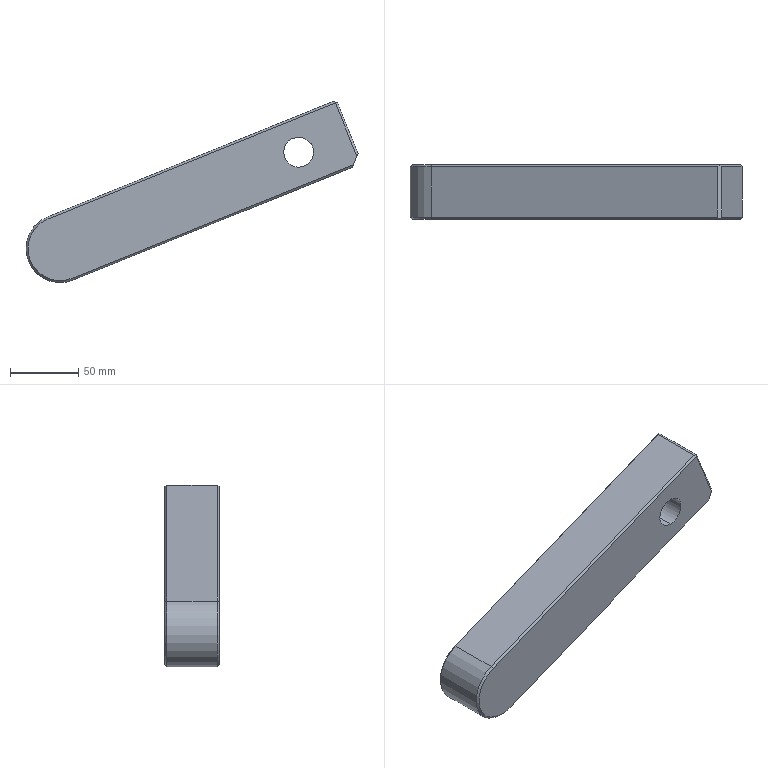Part | Creo | 1 solid | 21 faces | box 243.584 x 40 x 133.061 mm | volume 471581 mm3 | plane 14 | cylinder 5 | cone 2 | commonest cylinder face diameters 22 x2 31 x2 50 x1
STEP:
#1=CARTESIAN_POINT('',(93.939,390.,-84.108));
#2=VERTEX_POINT('',#1);
#3=CARTESIAN_POINT('',(-116.807,390.,-169.256));
#4=VERTEX_POINT('',#3);
#5=CARTESIAN_POINT('',(93.939,390.,-84.108));
#6=DIRECTION('',(-0.9272,0.,-0.3746));
#7=VECTOR('',#6,227.297);
#8=LINE('',#5,#7);
#9=EDGE_CURVE('',#2,#4,#8,.T.);
#10=ORIENTED_EDGE('',*,*,#9,.T.);
#11=CARTESIAN_POINT('',(-108.414,390.,-214.541));
#12=VERTEX_POINT('',#11);
#13=CARTESIAN_POINT('',(-108.004,390.,-191.044));
#14=DIRECTION('',(0.,1.,0.));
#15=DIRECTION('',(-0.01745,0.,-0.9998));
#16=AXIS2_PLACEMENT_3D('',#13,#14,#15);
#17=CIRCLE('',#16,23.5);
#18=EDGE_CURVE('',#12,#4,#17,.T.);
#19=ORIENTED_EDGE('',*,*,#18,.F.);
#20=CARTESIAN_POINT('',(-99.201,390.,-212.833));
#21=VERTEX_POINT('',#20);
#22=CARTESIAN_POINT('',(-108.004,390.,-191.044));
#23=DIRECTION('',(0.,1.,0.));
#24=DIRECTION('',(0.3746,0.,-0.9272));
#25=AXIS2_PLACEMENT_3D('',#22,#23,#24);
#26=CIRCLE('',#25,23.5);
#27=EDGE_CURVE('',#21,#12,#26,.T.);
#28=ORIENTED_EDGE('',*,*,#27,.F.);
#29=CARTESIAN_POINT('',(107.104,390.,-129.481));
#30=VERTEX_POINT('',#29);
#31=CARTESIAN_POINT('',(-99.201,390.,-212.833));
#32=DIRECTION('',(0.9272,0.,0.3746));
#33=VECTOR('',#32,222.507);
#34=LINE('',#31,#33);
#35=EDGE_CURVE('',#21,#30,#34,.T.);
#36=ORIENTED_EDGE('',*,*,#35,.T.);
#37=CARTESIAN_POINT('',(109.751,390.,-123.245));
#38=VERTEX_POINT('',#37);
#39=CARTESIAN_POINT('',(109.751,390.,-123.245));
#40=DIRECTION('',(-0.3907,0.,-0.9205));
#41=VECTOR('',#40,6.774);
#42=LINE('',#39,#41);
#43=EDGE_CURVE('',#38,#30,#42,.T.);
#44=ORIENTED_EDGE('',*,*,#43,.F.);
#45=CARTESIAN_POINT('',(109.751,390.,-123.245));
#46=DIRECTION('',(-0.3746,0.,0.9272));
#47=VECTOR('',#46,42.21);
#48=LINE('',#45,#47);
#49=EDGE_CURVE('',#38,#2,#48,.T.);
#50=ORIENTED_EDGE('',*,*,#49,.T.);
#51=EDGE_LOOP('',(#10,#19,#28,#36,#44,#50));
#52=FACE_OUTER_BOUND('',#51,.F.);
#53=CARTESIAN_POINT('',(67.046,390.,-135.82));
#54=VERTEX_POINT('',#53);
#55=CARTESIAN_POINT('',(67.316,390.,-104.822));
#56=VERTEX_POINT('',#55);
#57=CARTESIAN_POINT('',(67.046,390.,-120.32));
#58=DIRECTION('',(0.,-1.,0.));
#59=DIRECTION('',(0.,0.,-1.));
#60=AXIS2_PLACEMENT_3D('',#57,#58,#59);
#61=CIRCLE('',#60,15.5);
#62=EDGE_CURVE('',#54,#56,#61,.T.);
#63=ORIENTED_EDGE('',*,*,#62,.F.);
#64=CARTESIAN_POINT('',(66.775,390.,-135.817));
#65=VERTEX_POINT('',#64);
#66=CARTESIAN_POINT('',(67.046,390.,-120.32));
#67=DIRECTION('',(0.,-1.,0.));
#68=DIRECTION('',(-0.01745,0.,-0.9998));
#69=AXIS2_PLACEMENT_3D('',#66,#67,#68);
#70=CIRCLE('',#69,15.5);
#71=EDGE_CURVE('',#65,#54,#70,.T.);
#72=ORIENTED_EDGE('',*,*,#71,.F.);
#73=CARTESIAN_POINT('',(67.046,390.,-120.32));
#74=DIRECTION('',(0.,-1.,0.));
#75=DIRECTION('',(0.01745,0.,0.9998));
#76=AXIS2_PLACEMENT_3D('',#73,#74,#75);
#77=CIRCLE('',#76,15.5);
#78=EDGE_CURVE('',#56,#65,#77,.T.);
#79=ORIENTED_EDGE('',*,*,#78,.F.);
#80=EDGE_LOOP('',(#63,#72,#79));
#81=FACE_BOUND('',#80,.F.);
#82=CARTESIAN_POINT('',(343.725,390.,-2.208));
#83=DIRECTION('',(0.,1.,0.));
#84=DIRECTION('',(-0.01745,0.,-0.9998));
#85=AXIS2_PLACEMENT_3D('',#82,#83,#84);
#86=PLANE('',#85);
#87=ADVANCED_FACE('',(#52,#81),#86,.T.);
#88=CARTESIAN_POINT('',(94.157,389.605,-83.594));
#89=VERTEX_POINT('',#88);
#90=CARTESIAN_POINT('',(94.157,389.605,-83.594));
#91=DIRECTION('',(-0.319,0.5774,-0.7516));
#92=VECTOR('',#91,0.6844);
#93=LINE('',#90,#92);
#94=EDGE_CURVE('',#89,#2,#93,.T.);
#95=ORIENTED_EDGE('',*,*,#94,.F.);
#96=CARTESIAN_POINT('',(92.719,388.5,-82.984));
#97=VERTEX_POINT('',#96);
#98=CARTESIAN_POINT('',(92.719,388.5,-82.984));
#99=DIRECTION('',(0.7516,0.5774,-0.319));
#100=VECTOR('',#99,1.914);
#101=LINE('',#98,#100);
#102=EDGE_CURVE('',#97,#89,#101,.T.);
#103=ORIENTED_EDGE('',*,*,#102,.F.);
#104=CARTESIAN_POINT('',(-117.369,388.5,-167.865));
#105=VERTEX_POINT('',#104);
#106=CARTESIAN_POINT('',(-117.369,388.5,-167.865));
#107=DIRECTION('',(0.9272,0.,0.3746));
#108=VECTOR('',#107,226.588);
#109=LINE('',#106,#108);
#110=EDGE_CURVE('',#105,#97,#109,.T.);
#111=ORIENTED_EDGE('',*,*,#110,.F.);
#112=CARTESIAN_POINT('',(-116.807,390.,-169.256));
#113=DIRECTION('',(-0.2649,-0.7071,0.6556));
#114=VECTOR('',#113,2.121);
#115=LINE('',#112,#114);
#116=EDGE_CURVE('',#4,#105,#115,.T.);
#117=ORIENTED_EDGE('',*,*,#116,.F.);
#118=ORIENTED_EDGE('',*,*,#9,.F.);
#119=EDGE_LOOP('',(#95,#103,#111,#117,#118));
#120=FACE_OUTER_BOUND('',#119,.F.);
#121=CARTESIAN_POINT('',(2.704,389.25,-120.161));
#122=DIRECTION('',(-0.2649,0.7071,0.6556));
#123=DIRECTION('',(-0.01284,0.6773,-0.7356));
#124=AXIS2_PLACEMENT_3D('',#121,#122,#123);
#125=PLANE('',#124);
#126=ADVANCED_FACE('',(#120),#125,.T.);
#127=ORIENTED_EDGE('',*,*,#49,.F.);
#128=CARTESIAN_POINT('',(110.58,388.5,-121.292));
#129=VERTEX_POINT('',#128);
#130=CARTESIAN_POINT('',(110.58,388.5,-121.292));
#131=DIRECTION('',(-0.319,0.5774,-0.7516));
#132=VECTOR('',#131,2.598);
#133=LINE('',#130,#132);
#134=EDGE_CURVE('',#129,#38,#133,.T.);
#135=ORIENTED_EDGE('',*,*,#134,.F.);
#136=CARTESIAN_POINT('',(95.596,388.5,-84.205));
#137=VERTEX_POINT('',#136);
#138=CARTESIAN_POINT('',(95.596,388.5,-84.205));
#139=DIRECTION('',(0.3746,0.,-0.9272));
#140=VECTOR('',#139,40.);
#141=LINE('',#138,#140);
#142=EDGE_CURVE('',#137,#129,#141,.T.);
#143=ORIENTED_EDGE('',*,*,#142,.F.);
#144=CARTESIAN_POINT('',(94.157,389.605,-83.594));
#145=DIRECTION('',(0.7516,-0.5774,-0.319));
#146=VECTOR('',#145,1.914);
#147=LINE('',#144,#146);
#148=EDGE_CURVE('',#89,#137,#147,.T.);
#149=ORIENTED_EDGE('',*,*,#148,.F.);
#150=ORIENTED_EDGE('',*,*,#94,.T.);
#151=EDGE_LOOP('',(#127,#135,#143,#149,#150));
#152=FACE_OUTER_BOUND('',#151,.F.);
#153=CARTESIAN_POINT('',(102.393,389.25,-103.029));
#154=DIRECTION('',(0.6556,0.7071,0.2649));
#155=DIRECTION('',(-0.7356,0.6773,0.01284));
#156=AXIS2_PLACEMENT_3D('',#153,#154,#155);
#157=PLANE('',#156);
#158=ADVANCED_FACE('',(#152),#157,.T.);
#159=ORIENTED_EDGE('',*,*,#43,.T.);
#160=CARTESIAN_POINT('',(106.275,388.5,-131.433));
#161=VERTEX_POINT('',#160);
#162=CARTESIAN_POINT('',(107.104,390.,-129.481));
#163=DIRECTION('',(-0.319,-0.5774,-0.7516));
#164=VECTOR('',#163,2.598);
#165=LINE('',#162,#164);
#166=EDGE_CURVE('',#30,#161,#165,.T.);
#167=ORIENTED_EDGE('',*,*,#166,.T.);
#168=CARTESIAN_POINT('',(106.275,351.5,-131.433));
#169=VERTEX_POINT('',#168);
#170=CARTESIAN_POINT('',(106.275,351.5,-131.433));
#171=DIRECTION('',(0.,1.,0.));
#172=VECTOR('',#171,37.);
#173=LINE('',#170,#172);
#174=EDGE_CURVE('',#169,#161,#173,.T.);
#175=ORIENTED_EDGE('',*,*,#174,.F.);
#176=CARTESIAN_POINT('',(107.104,350.,-129.481));
#177=VERTEX_POINT('',#176);
#178=CARTESIAN_POINT('',(106.275,351.5,-131.433));
#179=DIRECTION('',(0.319,-0.5774,0.7516));
#180=VECTOR('',#179,2.598);
#181=LINE('',#178,#180);
#182=EDGE_CURVE('',#169,#177,#181,.T.);
#183=ORIENTED_EDGE('',*,*,#182,.T.);
#184=CARTESIAN_POINT('',(109.751,350.,-123.245));
#185=VERTEX_POINT('',#184);
#186=CARTESIAN_POINT('',(107.104,350.,-129.481));
#187=DIRECTION('',(0.3907,0.,0.9205));
#188=VECTOR('',#187,6.774);
#189=LINE('',#186,#188);
#190=EDGE_CURVE('',#177,#185,#189,.T.);
#191=ORIENTED_EDGE('',*,*,#190,.T.);
#192=CARTESIAN_POINT('',(110.58,351.5,-121.292));
#193=VERTEX_POINT('',#192);
#194=CARTESIAN_POINT('',(109.751,350.,-123.245));
#195=DIRECTION('',(0.319,0.5774,0.7516));
#196=VECTOR('',#195,2.598);
#197=LINE('',#194,#196);
#198=EDGE_CURVE('',#185,#193,#197,.T.);
#199=ORIENTED_EDGE('',*,*,#198,.T.);
#200=CARTESIAN_POINT('',(110.58,351.5,-121.292));
#201=DIRECTION('',(0.,1.,0.));
#202=VECTOR('',#201,37.);
#203=LINE('',#200,#202);
#204=EDGE_CURVE('',#193,#129,#203,.T.);
#205=ORIENTED_EDGE('',*,*,#204,.T.);
#206=ORIENTED_EDGE('',*,*,#134,.T.);
#207=EDGE_LOOP('',(#159,#167,#175,#183,#191,#199,#205,#206));
#208=FACE_OUTER_BOUND('',#207,.F.);
#209=CARTESIAN_POINT('',(109.199,370.,-124.546));
#210=DIRECTION('',(0.9205,0.,-0.3907));
#211=DIRECTION('',(0.3907,0.,0.9205));
#212=AXIS2_PLACEMENT_3D('',#209,#210,#211);
#213=PLANE('',#212);
#214=ADVANCED_FACE('',(#208),#213,.T.);
#215=CARTESIAN_POINT('',(-98.639,388.5,-214.224));
#216=VERTEX_POINT('',#215);
#217=CARTESIAN_POINT('',(106.275,388.5,-131.433));
#218=DIRECTION('',(-0.9272,0.,-0.3746));
#219=VECTOR('',#218,221.007);
#220=LINE('',#217,#219);
#221=EDGE_CURVE('',#161,#216,#220,.T.);
#222=ORIENTED_EDGE('',*,*,#221,.F.);
#223=ORIENTED_EDGE('',*,*,#166,.F.);
#224=ORIENTED_EDGE('',*,*,#35,.F.);
#225=CARTESIAN_POINT('',(-98.639,388.5,-214.224));
#226=DIRECTION('',(-0.2649,0.7071,0.6556));
#227=VECTOR('',#226,2.121);
#228=LINE('',#225,#227);
#229=EDGE_CURVE('',#216,#21,#228,.T.);
#230=ORIENTED_EDGE('',*,*,#229,.F.);
#231=EDGE_LOOP('',(#222,#223,#224,#230));
#232=FACE_OUTER_BOUND('',#231,.F.);
#233=CARTESIAN_POINT('',(20.872,389.25,-165.129));
#234=DIRECTION('',(0.2649,0.7071,-0.6556));
#235=DIRECTION('',(-0.01284,-0.6773,-0.7356));
#236=AXIS2_PLACEMENT_3D('',#233,#234,#235);
#237=PLANE('',#236);
#238=ADVANCED_FACE('',(#232),#237,.T.);
#239=ORIENTED_EDGE('',*,*,#174,.T.);
#240=ORIENTED_EDGE('',*,*,#221,.T.);
#241=CARTESIAN_POINT('',(-98.639,351.5,-214.224));
#242=VERTEX_POINT('',#241);
#243=CARTESIAN_POINT('',(-98.639,388.5,-214.224));
#244=DIRECTION('',(0.,-1.,0.));
#245=VECTOR('',#244,37.);
#246=LINE('',#243,#245);
#247=EDGE_CURVE('',#216,#242,#246,.T.);
#248=ORIENTED_EDGE('',*,*,#247,.T.);
#249=CARTESIAN_POINT('',(-98.639,351.5,-214.224));
#250=DIRECTION('',(0.9272,0.,0.3746));
#251=VECTOR('',#250,221.007);
#252=LINE('',#249,#251);
#253=EDGE_CURVE('',#242,#169,#252,.T.);
#254=ORIENTED_EDGE('',*,*,#253,.T.);
#255=EDGE_LOOP('',(#239,#240,#248,#254));
#256=FACE_OUTER_BOUND('',#255,.F.);
#257=CARTESIAN_POINT('',(145.859,350.,-115.44));
#258=DIRECTION('',(0.3746,0.,-0.9272));
#259=DIRECTION('',(0.9272,0.,0.3746));
#260=AXIS2_PLACEMENT_3D('',#257,#258,#259);
#261=PLANE('',#260);
#262=ADVANCED_FACE('',(#256),#261,.T.);
#263=ORIENTED_EDGE('',*,*,#247,.F.);
#264=CARTESIAN_POINT('',(-108.44,388.5,-216.041));
#265=VERTEX_POINT('',#264);
#266=CARTESIAN_POINT('',(-108.004,388.5,-191.044));
#267=DIRECTION('',(0.,1.,0.));
#268=DIRECTION('',(0.3746,0.,-0.9272));
#269=AXIS2_PLACEMENT_3D('',#266,#267,#268);
#270=CIRCLE('',#269,25.);
#271=EDGE_CURVE('',#216,#265,#270,.T.);
#272=ORIENTED_EDGE('',*,*,#271,.T.);
#273=CARTESIAN_POINT('',(-108.004,388.5,-191.044));
#274=DIRECTION('',(0.,1.,0.));
#275=DIRECTION('',(-0.01745,0.,-0.9998));
#276=AXIS2_PLACEMENT_3D('',#273,#274,#275);
#277=CIRCLE('',#276,25.);
#278=EDGE_CURVE('',#265,#105,#277,.T.);
#279=ORIENTED_EDGE('',*,*,#278,.T.);
#280=CARTESIAN_POINT('',(-117.369,351.5,-167.865));
#281=VERTEX_POINT('',#280);
#282=CARTESIAN_POINT('',(-117.369,351.5,-167.865));
#283=DIRECTION('',(0.,1.,0.));
#284=VECTOR('',#283,37.);
#285=LINE('',#282,#284);
#286=EDGE_CURVE('',#281,#105,#285,.T.);
#287=ORIENTED_EDGE('',*,*,#286,.F.);
#288=CARTESIAN_POINT('',(-108.44,351.5,-216.041));
#289=VERTEX_POINT('',#288);
#290=CARTESIAN_POINT('',(-108.004,351.5,-191.044));
#291=DIRECTION('',(0.,-1.,0.));
#292=DIRECTION('',(-0.3746,0.,0.9272));
#293=AXIS2_PLACEMENT_3D('',#290,#291,#292);
#294=CIRCLE('',#293,25.);
#295=EDGE_CURVE('',#281,#289,#294,.T.);
#296=ORIENTED_EDGE('',*,*,#295,.T.);
#297=CARTESIAN_POINT('',(-108.004,351.5,-191.044));
#298=DIRECTION('',(0.,-1.,0.));
#299=DIRECTION('',(-0.01745,0.,-0.9998));
#300=AXIS2_PLACEMENT_3D('',#297,#298,#299);
#301=CIRCLE('',#300,25.);
#302=EDGE_CURVE('',#289,#242,#301,.T.);
#303=ORIENTED_EDGE('',*,*,#302,.T.);
#304=EDGE_LOOP('',(#263,#272,#279,#287,#296,#303));
#305=FACE_OUTER_BOUND('',#304,.F.);
#306=CARTESIAN_POINT('',(-108.004,350.,-191.044));
#307=DIRECTION('',(0.,1.,0.));
#308=DIRECTION('',(-0.01745,0.,-0.9998));
#309=AXIS2_PLACEMENT_3D('',#306,#307,#308);
#310=CYLINDRICAL_SURFACE('',#309,25.);
#311=ADVANCED_FACE('',(#305),#310,.T.);
#312=ORIENTED_EDGE('',*,*,#229,.T.);
#313=ORIENTED_EDGE('',*,*,#27,.T.);
#314=ORIENTED_EDGE('',*,*,#18,.T.);
#315=ORIENTED_EDGE('',*,*,#116,.T.);
#316=ORIENTED_EDGE('',*,*,#278,.F.);
#317=ORIENTED_EDGE('',*,*,#271,.F.);
#318=EDGE_LOOP('',(#312,#313,#314,#315,#316,#317));
#319=FACE_OUTER_BOUND('',#318,.F.);
#320=CARTESIAN_POINT('',(-108.004,389.25,-191.044));
#321=DIRECTION('',(0.,-1.,0.));
#322=DIRECTION('',(0.01745,0.,0.9998));
#323=AXIS2_PLACEMENT_3D('',#320,#321,#322);
#324=CONICAL_SURFACE('',#323,24.25,45.);
#325=ADVANCED_FACE('',(#319),#324,.T.);
#326=ORIENTED_EDGE('',*,*,#286,.T.);
#327=ORIENTED_EDGE('',*,*,#110,.T.);
#328=CARTESIAN_POINT('',(92.719,351.5,-82.984));
#329=VERTEX_POINT('',#328);
#330=CARTESIAN_POINT('',(92.719,351.5,-82.984));
#331=DIRECTION('',(0.,1.,0.));
#332=VECTOR('',#331,37.);
#333=LINE('',#330,#332);
#334=EDGE_CURVE('',#329,#97,#333,.T.);
#335=ORIENTED_EDGE('',*,*,#334,.F.);
#336=CARTESIAN_POINT('',(92.719,351.5,-82.984));
#337=DIRECTION('',(-0.9272,0.,-0.3746));
#338=VECTOR('',#337,226.588);
#339=LINE('',#336,#338);
#340=EDGE_CURVE('',#329,#281,#339,.T.);
#341=ORIENTED_EDGE('',*,*,#340,.T.);
#342=EDGE_LOOP('',(#326,#327,#335,#341));
#343=FACE_OUTER_BOUND('',#342,.F.);
#344=CARTESIAN_POINT('',(-117.647,350.,-167.977));
#345=DIRECTION('',(-0.3746,0.,0.9272));
#346=DIRECTION('',(-0.9272,0.,-0.3746));
#347=AXIS2_PLACEMENT_3D('',#344,#345,#346);
#348=PLANE('',#347);
#349=ADVANCED_FACE('',(#343),#348,.T.);
#350=ORIENTED_EDGE('',*,*,#334,.T.);
#351=ORIENTED_EDGE('',*,*,#102,.T.);
#352=ORIENTED_EDGE('',*,*,#148,.T.);
#353=CARTESIAN_POINT('',(95.596,351.5,-84.205));
#354=VERTEX_POINT('',#353);
#355=CARTESIAN_POINT('',(95.596,351.5,-84.205));
#356=DIRECTION('',(0.,1.,0.));
#357=VECTOR('',#356,37.);
#358=LINE('',#355,#357);
#359=EDGE_CURVE('',#354,#137,#358,.T.);
#360=ORIENTED_EDGE('',*,*,#359,.F.);
#361=CARTESIAN_POINT('',(94.157,350.395,-83.594));
#362=VERTEX_POINT('',#361);
#363=CARTESIAN_POINT('',(95.596,351.5,-84.205));
#364=DIRECTION('',(-0.7516,-0.5774,0.319));
#365=VECTOR('',#364,1.914);
#366=LINE('',#363,#365);
#367=EDGE_CURVE('',#354,#362,#366,.T.);
#368=ORIENTED_EDGE('',*,*,#367,.T.);
#369=CARTESIAN_POINT('',(94.157,350.395,-83.594));
#370=DIRECTION('',(-0.7516,0.5774,0.319));
#371=VECTOR('',#370,1.914);
#372=LINE('',#369,#371);
#373=EDGE_CURVE('',#362,#329,#372,.T.);
#374=ORIENTED_EDGE('',*,*,#373,.T.);
#375=EDGE_LOOP('',(#350,#351,#352,#360,#368,#374));
#376=FACE_OUTER_BOUND('',#375,.F.);
#377=CARTESIAN_POINT('',(92.341,370.,-82.823));
#378=DIRECTION('',(0.3907,0.,0.9205));
#379=DIRECTION('',(-0.9205,0.,0.3907));
#380=AXIS2_PLACEMENT_3D('',#377,#378,#379);
#381=PLANE('',#380);
#382=ADVANCED_FACE('',(#376),#381,.T.);
#383=ORIENTED_EDGE('',*,*,#359,.T.);
#384=ORIENTED_EDGE('',*,*,#142,.T.);
#385=ORIENTED_EDGE('',*,*,#204,.F.);
#386=CARTESIAN_POINT('',(110.58,351.5,-121.292));
#387=DIRECTION('',(-0.3746,0.,0.9272));
#388=VECTOR('',#387,40.);
#389=LINE('',#386,#388);
#390=EDGE_CURVE('',#193,#354,#389,.T.);
#391=ORIENTED_EDGE('',*,*,#390,.T.);
#392=EDGE_LOOP('',(#383,#384,#385,#391));
#393=FACE_OUTER_BOUND('',#392,.F.);
#394=CARTESIAN_POINT('',(93.723,350.,-79.569));
#395=DIRECTION('',(0.9272,0.,0.3746));
#396=DIRECTION('',(-0.3746,0.,0.9272));
#397=AXIS2_PLACEMENT_3D('',#394,#395,#396);
#398=PLANE('',#397);
#399=ADVANCED_FACE('',(#393),#398,.T.);
#400=CARTESIAN_POINT('',(93.939,350.,-84.108));
#401=VERTEX_POINT('',#400);
#402=CARTESIAN_POINT('',(94.157,350.395,-83.594));
#403=DIRECTION('',(-0.319,-0.5774,-0.7516));
#404=VECTOR('',#403,0.6844);
#405=LINE('',#402,#404);
#406=EDGE_CURVE('',#362,#401,#405,.T.);
#407=ORIENTED_EDGE('',*,*,#406,.F.);
#408=ORIENTED_EDGE('',*,*,#367,.F.);
#409=ORIENTED_EDGE('',*,*,#390,.F.);
#410=ORIENTED_EDGE('',*,*,#198,.F.);
#411=CARTESIAN_POINT('',(93.939,350.,-84.108));
#412=DIRECTION('',(0.3746,0.,-0.9272));
#413=VECTOR('',#412,42.21);
#414=LINE('',#411,#413);
#415=EDGE_CURVE('',#401,#185,#414,.T.);
#416=ORIENTED_EDGE('',*,*,#415,.F.);
#417=EDGE_LOOP('',(#407,#408,#409,#410,#416));
#418=FACE_OUTER_BOUND('',#417,.F.);
#419=CARTESIAN_POINT('',(102.393,350.75,-103.029));
#420=DIRECTION('',(0.6556,-0.7071,0.2649));
#421=DIRECTION('',(0.7356,0.6773,-0.01284));
#422=AXIS2_PLACEMENT_3D('',#419,#420,#421);
#423=PLANE('',#422);
#424=ADVANCED_FACE('',(#418),#423,.T.);
#425=CARTESIAN_POINT('',(-116.807,350.,-169.256));
#426=VERTEX_POINT('',#425);
#427=CARTESIAN_POINT('',(-116.807,350.,-169.256));
#428=DIRECTION('',(0.9272,0.,0.3746));
#429=VECTOR('',#428,227.297);
#430=LINE('',#427,#429);
#431=EDGE_CURVE('',#426,#401,#430,.T.);
#432=ORIENTED_EDGE('',*,*,#431,.F.);
#433=CARTESIAN_POINT('',(-117.369,351.5,-167.865));
#434=DIRECTION('',(0.2649,-0.7071,-0.6556));
#435=VECTOR('',#434,2.121);
#436=LINE('',#433,#435);
#437=EDGE_CURVE('',#281,#426,#436,.T.);
#438=ORIENTED_EDGE('',*,*,#437,.F.);
#439=ORIENTED_EDGE('',*,*,#340,.F.);
#440=ORIENTED_EDGE('',*,*,#373,.F.);
#441=ORIENTED_EDGE('',*,*,#406,.T.);
#442=EDGE_LOOP('',(#432,#438,#439,#440,#441));
#443=FACE_OUTER_BOUND('',#442,.F.);
#444=CARTESIAN_POINT('',(2.704,350.75,-120.161));
#445=DIRECTION('',(-0.2649,-0.7071,0.6556));
#446=DIRECTION('',(0.01284,0.6773,0.7356));
#447=AXIS2_PLACEMENT_3D('',#444,#445,#446);
#448=PLANE('',#447);
#449=ADVANCED_FACE('',(#443),#448,.T.);
#450=ORIENTED_EDGE('',*,*,#190,.F.);
#451=CARTESIAN_POINT('',(-99.201,350.,-212.833));
#452=VERTEX_POINT('',#451);
#453=CARTESIAN_POINT('',(107.104,350.,-129.481));
#454=DIRECTION('',(-0.9272,0.,-0.3746));
#455=VECTOR('',#454,222.507);
#456=LINE('',#453,#455);
#457=EDGE_CURVE('',#177,#452,#456,.T.);
#458=ORIENTED_EDGE('',*,*,#457,.T.);
#459=CARTESIAN_POINT('',(-108.414,350.,-214.541));
#460=VERTEX_POINT('',#459);
#461=CARTESIAN_POINT('',(-108.004,350.,-191.044));
#462=DIRECTION('',(0.,-1.,0.));
#463=DIRECTION('',(-0.01745,0.,-0.9998));
#464=AXIS2_PLACEMENT_3D('',#461,#462,#463);
#465=CIRCLE('',#464,23.5);
#466=EDGE_CURVE('',#460,#452,#465,.T.);
#467=ORIENTED_EDGE('',*,*,#466,.F.);
#468=CARTESIAN_POINT('',(-108.004,350.,-191.044));
#469=DIRECTION('',(0.,-1.,0.));
#470=DIRECTION('',(-0.3746,0.,0.9272));
#471=AXIS2_PLACEMENT_3D('',#468,#469,#470);
#472=CIRCLE('',#471,23.5);
#473=EDGE_CURVE('',#426,#460,#472,.T.);
#474=ORIENTED_EDGE('',*,*,#473,.F.);
#475=ORIENTED_EDGE('',*,*,#431,.T.);
#476=ORIENTED_EDGE('',*,*,#415,.T.);
#477=EDGE_LOOP('',(#450,#458,#467,#474,#475,#476));
#478=FACE_OUTER_BOUND('',#477,.F.);
#479=CARTESIAN_POINT('',(66.854,350.,-131.318));
#480=VERTEX_POINT('',#479);
#481=CARTESIAN_POINT('',(67.046,350.,-131.32));
#482=VERTEX_POINT('',#481);
#483=CARTESIAN_POINT('',(67.046,350.,-120.32));
#484=DIRECTION('',(0.,-1.,0.));
#485=DIRECTION('',(-0.01745,0.,-0.9998));
#486=AXIS2_PLACEMENT_3D('',#483,#484,#485);
#487=CIRCLE('',#486,11.);
#488=EDGE_CURVE('',#480,#482,#487,.T.);
#489=ORIENTED_EDGE('',*,*,#488,.T.);
#490=CARTESIAN_POINT('',(67.238,350.,-109.321));
#491=VERTEX_POINT('',#490);
#492=CARTESIAN_POINT('',(67.046,350.,-120.32));
#493=DIRECTION('',(0.,1.,0.));
#494=DIRECTION('',(0.01745,0.,0.9998));
#495=AXIS2_PLACEMENT_3D('',#492,#493,#494);
#496=CIRCLE('',#495,11.);
#497=EDGE_CURVE('',#491,#482,#496,.T.);
#498=ORIENTED_EDGE('',*,*,#497,.F.);
#499=CARTESIAN_POINT('',(67.046,350.,-109.32));
#500=VERTEX_POINT('',#499);
#501=CARTESIAN_POINT('',(67.046,350.,-120.32));
#502=DIRECTION('',(0.,-1.,0.));
#503=DIRECTION('',(0.01745,0.,0.9998));
#504=AXIS2_PLACEMENT_3D('',#501,#502,#503);
#505=CIRCLE('',#504,11.);
#506=EDGE_CURVE('',#491,#500,#505,.T.);
#507=ORIENTED_EDGE('',*,*,#506,.T.);
#508=CARTESIAN_POINT('',(67.046,350.,-120.32));
#509=DIRECTION('',(0.,1.,0.));
#510=DIRECTION('',(-0.01745,0.,-0.9998));
#511=AXIS2_PLACEMENT_3D('',#508,#509,#510);
#512=CIRCLE('',#511,11.);
#513=EDGE_CURVE('',#480,#500,#512,.T.);
#514=ORIENTED_EDGE('',*,*,#513,.F.);
#515=EDGE_LOOP('',(#489,#498,#507,#514));
#516=FACE_BOUND('',#515,.F.);
#517=CARTESIAN_POINT('',(343.725,350.,-2.208));
#518=DIRECTION('',(0.,1.,0.));
#519=DIRECTION('',(-0.01745,0.,-0.9998));
#520=AXIS2_PLACEMENT_3D('',#517,#518,#519);
#521=PLANE('',#520);
#522=ADVANCED_FACE('',(#478,#516),#521,.F.);
#523=ORIENTED_EDGE('',*,*,#497,.T.);
#524=ORIENTED_EDGE('',*,*,#488,.F.);
#525=CARTESIAN_POINT('',(66.854,370.,-131.318));
#526=VERTEX_POINT('',#525);
#527=CARTESIAN_POINT('',(66.854,350.,-131.318));
#528=DIRECTION('',(0.,1.,0.));
#529=VECTOR('',#528,20.);
#530=LINE('',#527,#529);
#531=EDGE_CURVE('',#480,#526,#530,.T.);
#532=ORIENTED_EDGE('',*,*,#531,.T.);
#533=CARTESIAN_POINT('',(68.196,370.,-109.38));
#534=VERTEX_POINT('',#533);
#535=CARTESIAN_POINT('',(67.046,370.,-120.32));
#536=DIRECTION('',(0.,-1.,0.));
#537=DIRECTION('',(-0.01745,0.,-0.9998));
#538=AXIS2_PLACEMENT_3D('',#535,#536,#537);
#539=CIRCLE('',#538,11.);
#540=EDGE_CURVE('',#526,#534,#539,.T.);
#541=ORIENTED_EDGE('',*,*,#540,.T.);
#542=CARTESIAN_POINT('',(67.238,370.,-109.321));
#543=VERTEX_POINT('',#542);
#544=CARTESIAN_POINT('',(67.046,370.,-120.32));
#545=DIRECTION('',(0.,-1.,0.));
#546=DIRECTION('',(0.1045,0.,0.9945));
#547=AXIS2_PLACEMENT_3D('',#544,#545,#546);
#548=CIRCLE('',#547,11.);
#549=EDGE_CURVE('',#534,#543,#548,.T.);
#550=ORIENTED_EDGE('',*,*,#549,.T.);
#551=CARTESIAN_POINT('',(67.238,350.,-109.321));
#552=DIRECTION('',(0.,1.,0.));
#553=VECTOR('',#552,20.);
#554=LINE('',#551,#553);
#555=EDGE_CURVE('',#491,#543,#554,.T.);
#556=ORIENTED_EDGE('',*,*,#555,.F.);
#557=EDGE_LOOP('',(#523,#524,#532,#541,#550,#556));
#558=FACE_OUTER_BOUND('',#557,.F.);
#559=CARTESIAN_POINT('',(67.046,341.,-120.32));
#560=DIRECTION('',(0.,1.,0.));
#561=DIRECTION('',(-0.01745,0.,-0.9998));
#562=AXIS2_PLACEMENT_3D('',#559,#560,#561);
#563=CYLINDRICAL_SURFACE('',#562,11.);
#564=ADVANCED_FACE('',(#558),#563,.F.);
#565=ORIENTED_EDGE('',*,*,#506,.F.);
#566=ORIENTED_EDGE('',*,*,#555,.T.);
#567=CARTESIAN_POINT('',(67.046,370.,-120.32));
#568=DIRECTION('',(0.,-1.,0.));
#569=DIRECTION('',(0.01745,0.,0.9998));
#570=AXIS2_PLACEMENT_3D('',#567,#568,#569);
#571=CIRCLE('',#570,11.);
#572=EDGE_CURVE('',#543,#526,#571,.T.);
#573=ORIENTED_EDGE('',*,*,#572,.T.);
#574=ORIENTED_EDGE('',*,*,#531,.F.);
#575=ORIENTED_EDGE('',*,*,#513,.T.);
#576=EDGE_LOOP('',(#565,#566,#573,#574,#575));
#577=FACE_OUTER_BOUND('',#576,.F.);
#578=CARTESIAN_POINT('',(67.046,341.,-120.32));
#579=DIRECTION('',(0.,1.,0.));
#580=DIRECTION('',(-0.01745,0.,-0.9998));
#581=AXIS2_PLACEMENT_3D('',#578,#579,#580);
#582=CYLINDRICAL_SURFACE('',#581,11.);
#583=ADVANCED_FACE('',(#577),#582,.F.);
#584=CARTESIAN_POINT('',(67.046,370.,-135.82));
#585=VERTEX_POINT('',#584);
#586=CARTESIAN_POINT('',(66.775,370.,-135.817));
#587=VERTEX_POINT('',#586);
#588=CARTESIAN_POINT('',(67.046,370.,-120.32));
#589=DIRECTION('',(0.,1.,0.));
#590=DIRECTION('',(0.,0.,-1.));
#591=AXIS2_PLACEMENT_3D('',#588,#589,#590);
#592=CIRCLE('',#591,15.5);
#593=EDGE_CURVE('',#585,#587,#592,.T.);
#594=ORIENTED_EDGE('',*,*,#593,.F.);
#595=CARTESIAN_POINT('',(67.316,370.,-104.822));
#596=VERTEX_POINT('',#595);
#597=CARTESIAN_POINT('',(67.046,370.,-120.32));
#598=DIRECTION('',(0.,1.,0.));
#599=DIRECTION('',(0.01745,0.,0.9998));
#600=AXIS2_PLACEMENT_3D('',#597,#598,#599);
#601=CIRCLE('',#600,15.5);
#602=EDGE_CURVE('',#596,#585,#601,.T.);
#603=ORIENTED_EDGE('',*,*,#602,.F.);
#604=CARTESIAN_POINT('',(67.046,370.,-120.32));
#605=DIRECTION('',(0.,1.,0.));
#606=DIRECTION('',(-0.01745,0.,-0.9998));
#607=AXIS2_PLACEMENT_3D('',#604,#605,#606);
#608=CIRCLE('',#607,15.5);
#609=EDGE_CURVE('',#587,#596,#608,.T.);
#610=ORIENTED_EDGE('',*,*,#609,.F.);
#611=EDGE_LOOP('',(#594,#603,#610));
#612=FACE_OUTER_BOUND('',#611,.F.);
#613=ORIENTED_EDGE('',*,*,#549,.F.);
#614=ORIENTED_EDGE('',*,*,#540,.F.);
#615=ORIENTED_EDGE('',*,*,#572,.F.);
#616=EDGE_LOOP('',(#613,#614,#615));
#617=FACE_BOUND('',#616,.F.);
#618=CARTESIAN_POINT('',(13.059,370.,16.573));
#619=DIRECTION('',(0.,1.,0.));
#620=DIRECTION('',(-0.01745,0.,-0.9998));
#621=AXIS2_PLACEMENT_3D('',#618,#619,#620);
#622=PLANE('',#621);
#623=ADVANCED_FACE('',(#612,#617),#622,.T.);
#624=ORIENTED_EDGE('',*,*,#71,.T.);
#625=ORIENTED_EDGE('',*,*,#62,.T.);
#626=CARTESIAN_POINT('',(67.316,370.,-104.822));
#627=DIRECTION('',(0.,1.,0.));
#628=VECTOR('',#627,20.);
#629=LINE('',#626,#628);
#630=EDGE_CURVE('',#596,#56,#629,.T.);
#631=ORIENTED_EDGE('',*,*,#630,.F.);
#632=ORIENTED_EDGE('',*,*,#602,.T.);
#633=ORIENTED_EDGE('',*,*,#593,.T.);
#634=CARTESIAN_POINT('',(66.775,370.,-135.817));
#635=DIRECTION('',(0.,1.,0.));
#636=VECTOR('',#635,20.);
#637=LINE('',#634,#636);
#638=EDGE_CURVE('',#587,#65,#637,.T.);
#639=ORIENTED_EDGE('',*,*,#638,.T.);
#640=EDGE_LOOP('',(#624,#625,#631,#632,#633,#639));
#641=FACE_OUTER_BOUND('',#640,.F.);
#642=CARTESIAN_POINT('',(67.046,371.,-120.32));
#643=DIRECTION('',(0.,1.,0.));
#644=DIRECTION('',(-0.01745,0.,-0.9998));
#645=AXIS2_PLACEMENT_3D('',#642,#643,#644);
#646=CYLINDRICAL_SURFACE('',#645,15.5);
#647=ADVANCED_FACE('',(#641),#646,.F.);
#648=ORIENTED_EDGE('',*,*,#78,.T.);
#649=ORIENTED_EDGE('',*,*,#638,.F.);
#650=ORIENTED_EDGE('',*,*,#609,.T.);
#651=ORIENTED_EDGE('',*,*,#630,.T.);
#652=EDGE_LOOP('',(#648,#649,#650,#651));
#653=FACE_OUTER_BOUND('',#652,.F.);
#654=CARTESIAN_POINT('',(67.046,371.,-120.32));
#655=DIRECTION('',(0.,1.,0.));
#656=DIRECTION('',(-0.01745,0.,-0.9998));
#657=AXIS2_PLACEMENT_3D('',#654,#655,#656);
#658=CYLINDRICAL_SURFACE('',#657,15.5);
#659=ADVANCED_FACE('',(#653),#658,.F.);
#660=ORIENTED_EDGE('',*,*,#457,.F.);
#661=ORIENTED_EDGE('',*,*,#182,.F.);
#662=ORIENTED_EDGE('',*,*,#253,.F.);
#663=CARTESIAN_POINT('',(-99.201,350.,-212.833));
#664=DIRECTION('',(0.2649,0.7071,-0.6556));
#665=VECTOR('',#664,2.121);
#666=LINE('',#663,#665);
#667=EDGE_CURVE('',#452,#242,#666,.T.);
#668=ORIENTED_EDGE('',*,*,#667,.F.);
#669=EDGE_LOOP('',(#660,#661,#662,#668));
#670=FACE_OUTER_BOUND('',#669,.F.);
#671=CARTESIAN_POINT('',(20.872,350.75,-165.129));
#672=DIRECTION('',(0.2649,-0.7071,-0.6556));
#673=DIRECTION('',(0.01284,-0.6773,0.7356));
#674=AXIS2_PLACEMENT_3D('',#671,#672,#673);
#675=PLANE('',#674);
#676=ADVANCED_FACE('',(#670),#675,.T.);
#677=ORIENTED_EDGE('',*,*,#437,.T.);
#678=ORIENTED_EDGE('',*,*,#473,.T.);
#679=ORIENTED_EDGE('',*,*,#466,.T.);
#680=ORIENTED_EDGE('',*,*,#667,.T.);
#681=ORIENTED_EDGE('',*,*,#302,.F.);
#682=ORIENTED_EDGE('',*,*,#295,.F.);
#683=EDGE_LOOP('',(#677,#678,#679,#680,#681,#682));
#684=FACE_OUTER_BOUND('',#683,.F.);
#685=CARTESIAN_POINT('',(-108.004,350.75,-191.044));
#686=DIRECTION('',(0.,1.,0.));
#687=DIRECTION('',(-0.01745,0.,-0.9998));
#688=AXIS2_PLACEMENT_3D('',#685,#686,#687);
#689=CONICAL_SURFACE('',#688,24.25,45.);
#690=ADVANCED_FACE('',(#684),#689,.T.);
#691=CLOSED_SHELL('',(#87,#126,#158,#214,#238,#262,#311,#325,#349,#382,#399,#424,#449,#522,#564,#583,#623,#647,#659,#676,#690));
#692=MANIFOLD_SOLID_BREP('',#691);
#693=(LENGTH_UNIT()NAMED_UNIT(*)SI_UNIT(.MILLI.,.METRE.));
#694=UNCERTAINTY_MEASURE_WITH_UNIT(LENGTH_MEASURE(0.03084),#693,'','');
#695=(NAMED_UNIT(*)PLANE_ANGLE_UNIT()SI_UNIT($,.RADIAN.));
#696=PLANE_ANGLE_MEASURE_WITH_UNIT(PLANE_ANGLE_MEASURE(0.01745),#695);
#697=(CONVERSION_BASED_UNIT('DEGREE',#696)NAMED_UNIT(*)PLANE_ANGLE_UNIT());
#698=(NAMED_UNIT(*)SI_UNIT($,.STERADIAN.)SOLID_ANGLE_UNIT());
#699=(GEOMETRIC_REPRESENTATION_CONTEXT(3)GLOBAL_UNCERTAINTY_ASSIGNED_CONTEXT((#694))GLOBAL_UNIT_ASSIGNED_CONTEXT((#693,#697,#698))REPRESENTATION_CONTEXT('',''));
#700=ADVANCED_BREP_SHAPE_REPRESENTATION('',(#692),#699);